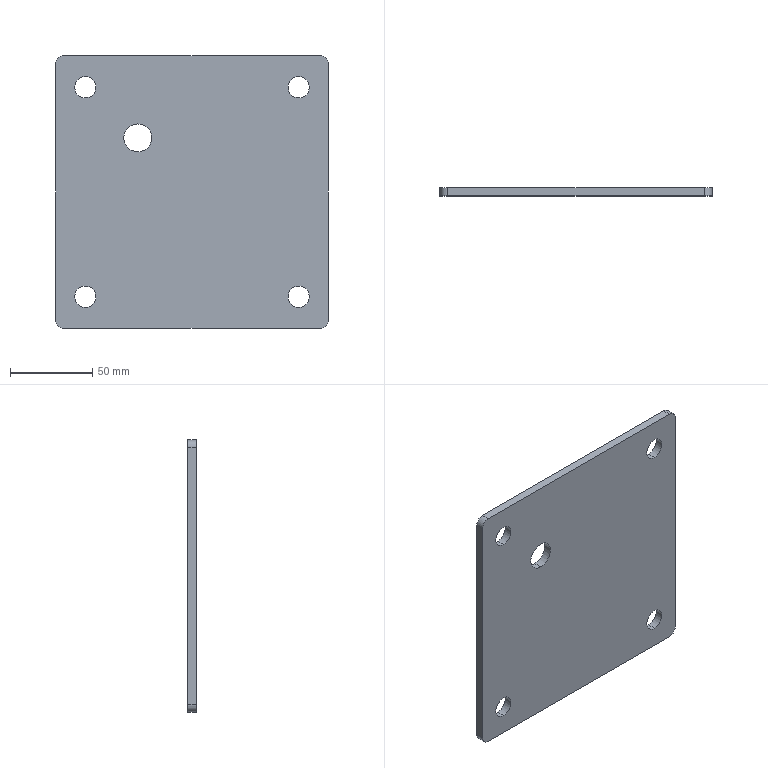Part | SolidWorks | features BaseBody 1 | 1 solid | 20 faces | box 166 x 5 x 166 mm | volume 133883 mm3 | cylinder 14 | plane 6 | commonest cylinder face diameters 13 x8 10 x4 17 x2
STEP:
#1=CARTESIAN_POINT('',(-33.,0.,24.5));
#2=VERTEX_POINT('',#1);
#3=CARTESIAN_POINT('',(-33.,0.,41.5));
#4=VERTEX_POINT('',#3);
#5=CARTESIAN_POINT('',(-33.,0.,33.));
#6=DIRECTION('',(0.,1.,0.));
#7=DIRECTION('',(0.,0.,1.));
#8=AXIS2_PLACEMENT_3D('',#5,#6,#7);
#9=CIRCLE('',#8,8.5);
#10=EDGE_CURVE('',#2,#4,#9,.T.);
#11=ORIENTED_EDGE('',*,*,#10,.F.);
#12=CARTESIAN_POINT('',(-33.,5.,24.5));
#13=VERTEX_POINT('',#12);
#14=CARTESIAN_POINT('',(-33.,1.,24.5));
#15=DIRECTION('',(0.,1.,0.));
#16=VECTOR('',#15,1000.);
#17=LINE('',#14,#16);
#18=EDGE_CURVE('',#2,#13,#17,.T.);
#19=ORIENTED_EDGE('',*,*,#18,.T.);
#20=CARTESIAN_POINT('',(-33.,5.,41.5));
#21=VERTEX_POINT('',#20);
#22=CARTESIAN_POINT('',(-33.,5.,33.));
#23=DIRECTION('',(0.,-1.,0.));
#24=DIRECTION('',(0.,0.,1.));
#25=AXIS2_PLACEMENT_3D('',#22,#23,#24);
#26=CIRCLE('',#25,8.5);
#27=EDGE_CURVE('',#21,#13,#26,.T.);
#28=ORIENTED_EDGE('',*,*,#27,.F.);
#29=CARTESIAN_POINT('',(-33.,1.,41.5));
#30=DIRECTION('',(0.,1.,0.));
#31=VECTOR('',#30,1000.);
#32=LINE('',#29,#31);
#33=EDGE_CURVE('',#4,#21,#32,.T.);
#34=ORIENTED_EDGE('',*,*,#33,.F.);
#35=EDGE_LOOP('',(#11,#19,#28,#34));
#36=FACE_OUTER_BOUND('',#35,.T.);
#37=CARTESIAN_POINT('',(-33.,1.,33.));
#38=DIRECTION('',(0.,1.,0.));
#39=DIRECTION('',(0.,0.,1.));
#40=AXIS2_PLACEMENT_3D('',#37,#38,#39);
#41=CYLINDRICAL_SURFACE('',#40,8.5);
#42=ADVANCED_FACE('',(#36),#41,.F.);
#43=CARTESIAN_POINT('',(-65.,0.,-70.262));
#44=VERTEX_POINT('',#43);
#45=CARTESIAN_POINT('',(-65.,0.,-57.262));
#46=VERTEX_POINT('',#45);
#47=CARTESIAN_POINT('',(-65.,0.,-63.762));
#48=DIRECTION('',(0.,1.,0.));
#49=DIRECTION('',(0.,0.,1.));
#50=AXIS2_PLACEMENT_3D('',#47,#48,#49);
#51=CIRCLE('',#50,6.5);
#52=EDGE_CURVE('',#44,#46,#51,.T.);
#53=ORIENTED_EDGE('',*,*,#52,.F.);
#54=CARTESIAN_POINT('',(-65.,5.,-70.262));
#55=VERTEX_POINT('',#54);
#56=CARTESIAN_POINT('',(-65.,-229.813,-70.262));
#57=DIRECTION('',(0.,1.,0.));
#58=VECTOR('',#57,1000.);
#59=LINE('',#56,#58);
#60=EDGE_CURVE('',#44,#55,#59,.T.);
#61=ORIENTED_EDGE('',*,*,#60,.T.);
#62=CARTESIAN_POINT('',(-65.,5.,-57.262));
#63=VERTEX_POINT('',#62);
#64=CARTESIAN_POINT('',(-65.,5.,-63.762));
#65=DIRECTION('',(0.,-1.,0.));
#66=DIRECTION('',(0.,0.,1.));
#67=AXIS2_PLACEMENT_3D('',#64,#65,#66);
#68=CIRCLE('',#67,6.5);
#69=EDGE_CURVE('',#63,#55,#68,.T.);
#70=ORIENTED_EDGE('',*,*,#69,.F.);
#71=CARTESIAN_POINT('',(-65.,-229.813,-57.262));
#72=DIRECTION('',(0.,1.,0.));
#73=VECTOR('',#72,1000.);
#74=LINE('',#71,#73);
#75=EDGE_CURVE('',#46,#63,#74,.T.);
#76=ORIENTED_EDGE('',*,*,#75,.F.);
#77=EDGE_LOOP('',(#53,#61,#70,#76));
#78=FACE_OUTER_BOUND('',#77,.T.);
#79=CARTESIAN_POINT('',(-65.,-229.813,-63.762));
#80=DIRECTION('',(0.,1.,0.));
#81=DIRECTION('',(0.,0.,1.));
#82=AXIS2_PLACEMENT_3D('',#79,#80,#81);
#83=CYLINDRICAL_SURFACE('',#82,6.5);
#84=ADVANCED_FACE('',(#78),#83,.F.);
#85=CARTESIAN_POINT('',(65.,0.,57.262));
#86=VERTEX_POINT('',#85);
#87=CARTESIAN_POINT('',(65.,0.,70.262));
#88=VERTEX_POINT('',#87);
#89=CARTESIAN_POINT('',(65.,0.,63.762));
#90=DIRECTION('',(0.,1.,0.));
#91=DIRECTION('',(0.,0.,1.));
#92=AXIS2_PLACEMENT_3D('',#89,#90,#91);
#93=CIRCLE('',#92,6.5);
#94=EDGE_CURVE('',#86,#88,#93,.T.);
#95=ORIENTED_EDGE('',*,*,#94,.F.);
#96=CARTESIAN_POINT('',(65.,5.,57.262));
#97=VERTEX_POINT('',#96);
#98=CARTESIAN_POINT('',(65.,-229.813,57.262));
#99=DIRECTION('',(0.,1.,0.));
#100=VECTOR('',#99,1000.);
#101=LINE('',#98,#100);
#102=EDGE_CURVE('',#86,#97,#101,.T.);
#103=ORIENTED_EDGE('',*,*,#102,.T.);
#104=CARTESIAN_POINT('',(65.,5.,70.262));
#105=VERTEX_POINT('',#104);
#106=CARTESIAN_POINT('',(65.,5.,63.762));
#107=DIRECTION('',(0.,-1.,0.));
#108=DIRECTION('',(0.,0.,1.));
#109=AXIS2_PLACEMENT_3D('',#106,#107,#108);
#110=CIRCLE('',#109,6.5);
#111=EDGE_CURVE('',#105,#97,#110,.T.);
#112=ORIENTED_EDGE('',*,*,#111,.F.);
#113=CARTESIAN_POINT('',(65.,-229.813,70.262));
#114=DIRECTION('',(0.,1.,0.));
#115=VECTOR('',#114,1000.);
#116=LINE('',#113,#115);
#117=EDGE_CURVE('',#88,#105,#116,.T.);
#118=ORIENTED_EDGE('',*,*,#117,.F.);
#119=EDGE_LOOP('',(#95,#103,#112,#118));
#120=FACE_OUTER_BOUND('',#119,.T.);
#121=CARTESIAN_POINT('',(65.,-229.813,63.762));
#122=DIRECTION('',(0.,1.,0.));
#123=DIRECTION('',(0.,0.,1.));
#124=AXIS2_PLACEMENT_3D('',#121,#122,#123);
#125=CYLINDRICAL_SURFACE('',#124,6.5);
#126=ADVANCED_FACE('',(#120),#125,.F.);
#127=CARTESIAN_POINT('',(65.,0.,-70.262));
#128=VERTEX_POINT('',#127);
#129=CARTESIAN_POINT('',(65.,0.,-57.262));
#130=VERTEX_POINT('',#129);
#131=CARTESIAN_POINT('',(65.,0.,-63.762));
#132=DIRECTION('',(0.,1.,0.));
#133=DIRECTION('',(0.,0.,1.));
#134=AXIS2_PLACEMENT_3D('',#131,#132,#133);
#135=CIRCLE('',#134,6.5);
#136=EDGE_CURVE('',#128,#130,#135,.T.);
#137=ORIENTED_EDGE('',*,*,#136,.F.);
#138=CARTESIAN_POINT('',(65.,5.,-70.262));
#139=VERTEX_POINT('',#138);
#140=CARTESIAN_POINT('',(65.,-229.813,-70.262));
#141=DIRECTION('',(0.,1.,0.));
#142=VECTOR('',#141,1000.);
#143=LINE('',#140,#142);
#144=EDGE_CURVE('',#128,#139,#143,.T.);
#145=ORIENTED_EDGE('',*,*,#144,.T.);
#146=CARTESIAN_POINT('',(65.,5.,-57.262));
#147=VERTEX_POINT('',#146);
#148=CARTESIAN_POINT('',(65.,5.,-63.762));
#149=DIRECTION('',(0.,-1.,0.));
#150=DIRECTION('',(0.,0.,1.));
#151=AXIS2_PLACEMENT_3D('',#148,#149,#150);
#152=CIRCLE('',#151,6.5);
#153=EDGE_CURVE('',#147,#139,#152,.T.);
#154=ORIENTED_EDGE('',*,*,#153,.F.);
#155=CARTESIAN_POINT('',(65.,-229.813,-57.262));
#156=DIRECTION('',(0.,1.,0.));
#157=VECTOR('',#156,1000.);
#158=LINE('',#155,#157);
#159=EDGE_CURVE('',#130,#147,#158,.T.);
#160=ORIENTED_EDGE('',*,*,#159,.F.);
#161=EDGE_LOOP('',(#137,#145,#154,#160));
#162=FACE_OUTER_BOUND('',#161,.T.);
#163=CARTESIAN_POINT('',(65.,-229.813,-63.762));
#164=DIRECTION('',(0.,1.,0.));
#165=DIRECTION('',(0.,0.,1.));
#166=AXIS2_PLACEMENT_3D('',#163,#164,#165);
#167=CYLINDRICAL_SURFACE('',#166,6.5);
#168=ADVANCED_FACE('',(#162),#167,.F.);
#169=CARTESIAN_POINT('',(-65.,0.,57.262));
#170=VERTEX_POINT('',#169);
#171=CARTESIAN_POINT('',(-65.,0.,70.262));
#172=VERTEX_POINT('',#171);
#173=CARTESIAN_POINT('',(-65.,0.,63.762));
#174=DIRECTION('',(0.,1.,0.));
#175=DIRECTION('',(0.,0.,1.));
#176=AXIS2_PLACEMENT_3D('',#173,#174,#175);
#177=CIRCLE('',#176,6.5);
#178=EDGE_CURVE('',#170,#172,#177,.T.);
#179=ORIENTED_EDGE('',*,*,#178,.F.);
#180=CARTESIAN_POINT('',(-65.,5.,57.262));
#181=VERTEX_POINT('',#180);
#182=CARTESIAN_POINT('',(-65.,-229.813,57.262));
#183=DIRECTION('',(0.,1.,0.));
#184=VECTOR('',#183,1000.);
#185=LINE('',#182,#184);
#186=EDGE_CURVE('',#170,#181,#185,.T.);
#187=ORIENTED_EDGE('',*,*,#186,.T.);
#188=CARTESIAN_POINT('',(-65.,5.,70.262));
#189=VERTEX_POINT('',#188);
#190=CARTESIAN_POINT('',(-65.,5.,63.762));
#191=DIRECTION('',(0.,-1.,0.));
#192=DIRECTION('',(0.,0.,1.));
#193=AXIS2_PLACEMENT_3D('',#190,#191,#192);
#194=CIRCLE('',#193,6.5);
#195=EDGE_CURVE('',#189,#181,#194,.T.);
#196=ORIENTED_EDGE('',*,*,#195,.F.);
#197=CARTESIAN_POINT('',(-65.,-229.813,70.262));
#198=DIRECTION('',(0.,1.,0.));
#199=VECTOR('',#198,1000.);
#200=LINE('',#197,#199);
#201=EDGE_CURVE('',#172,#189,#200,.T.);
#202=ORIENTED_EDGE('',*,*,#201,.F.);
#203=EDGE_LOOP('',(#179,#187,#196,#202));
#204=FACE_OUTER_BOUND('',#203,.T.);
#205=CARTESIAN_POINT('',(-65.,-229.813,63.762));
#206=DIRECTION('',(0.,1.,0.));
#207=DIRECTION('',(0.,0.,1.));
#208=AXIS2_PLACEMENT_3D('',#205,#206,#207);
#209=CYLINDRICAL_SURFACE('',#208,6.5);
#210=ADVANCED_FACE('',(#204),#209,.F.);
#211=ORIENTED_EDGE('',*,*,#27,.T.);
#212=CARTESIAN_POINT('',(-33.,5.,33.));
#213=DIRECTION('',(0.,-1.,0.));
#214=DIRECTION('',(0.,0.,1.));
#215=AXIS2_PLACEMENT_3D('',#212,#213,#214);
#216=CIRCLE('',#215,8.5);
#217=EDGE_CURVE('',#13,#21,#216,.T.);
#218=ORIENTED_EDGE('',*,*,#217,.T.);
#219=EDGE_LOOP('',(#211,#218));
#220=FACE_BOUND('',#219,.T.);
#221=ORIENTED_EDGE('',*,*,#69,.T.);
#222=CARTESIAN_POINT('',(-65.,5.,-63.762));
#223=DIRECTION('',(0.,-1.,0.));
#224=DIRECTION('',(0.,0.,1.));
#225=AXIS2_PLACEMENT_3D('',#222,#223,#224);
#226=CIRCLE('',#225,6.5);
#227=EDGE_CURVE('',#55,#63,#226,.T.);
#228=ORIENTED_EDGE('',*,*,#227,.T.);
#229=EDGE_LOOP('',(#221,#228));
#230=FACE_BOUND('',#229,.T.);
#231=ORIENTED_EDGE('',*,*,#111,.T.);
#232=CARTESIAN_POINT('',(65.,5.,63.762));
#233=DIRECTION('',(0.,-1.,0.));
#234=DIRECTION('',(0.,0.,1.));
#235=AXIS2_PLACEMENT_3D('',#232,#233,#234);
#236=CIRCLE('',#235,6.5);
#237=EDGE_CURVE('',#97,#105,#236,.T.);
#238=ORIENTED_EDGE('',*,*,#237,.T.);
#239=EDGE_LOOP('',(#231,#238));
#240=FACE_BOUND('',#239,.T.);
#241=ORIENTED_EDGE('',*,*,#153,.T.);
#242=CARTESIAN_POINT('',(65.,5.,-63.762));
#243=DIRECTION('',(0.,-1.,0.));
#244=DIRECTION('',(0.,0.,1.));
#245=AXIS2_PLACEMENT_3D('',#242,#243,#244);
#246=CIRCLE('',#245,6.5);
#247=EDGE_CURVE('',#139,#147,#246,.T.);
#248=ORIENTED_EDGE('',*,*,#247,.T.);
#249=EDGE_LOOP('',(#241,#248));
#250=FACE_BOUND('',#249,.T.);
#251=ORIENTED_EDGE('',*,*,#195,.T.);
#252=CARTESIAN_POINT('',(-65.,5.,63.762));
#253=DIRECTION('',(0.,-1.,0.));
#254=DIRECTION('',(0.,0.,1.));
#255=AXIS2_PLACEMENT_3D('',#252,#253,#254);
#256=CIRCLE('',#255,6.5);
#257=EDGE_CURVE('',#181,#189,#256,.T.);
#258=ORIENTED_EDGE('',*,*,#257,.T.);
#259=EDGE_LOOP('',(#251,#258));
#260=FACE_BOUND('',#259,.T.);
#261=CARTESIAN_POINT('',(-78.,5.,-83.));
#262=VERTEX_POINT('',#261);
#263=CARTESIAN_POINT('',(-83.,5.,-78.));
#264=VERTEX_POINT('',#263);
#265=CARTESIAN_POINT('',(-78.,5.,-78.));
#266=DIRECTION('',(0.,1.,0.));
#267=DIRECTION('',(0.,0.,1.));
#268=AXIS2_PLACEMENT_3D('',#265,#266,#267);
#269=CIRCLE('',#268,5.);
#270=EDGE_CURVE('',#262,#264,#269,.T.);
#271=ORIENTED_EDGE('',*,*,#270,.T.);
#272=CARTESIAN_POINT('',(-83.,5.,78.));
#273=VERTEX_POINT('',#272);
#274=CARTESIAN_POINT('',(-83.,5.,0.));
#275=DIRECTION('',(0.,0.,1.));
#276=VECTOR('',#275,1000.);
#277=LINE('',#274,#276);
#278=EDGE_CURVE('',#264,#273,#277,.T.);
#279=ORIENTED_EDGE('',*,*,#278,.T.);
#280=CARTESIAN_POINT('',(-78.,5.,83.));
#281=VERTEX_POINT('',#280);
#282=CARTESIAN_POINT('',(-78.,5.,78.));
#283=DIRECTION('',(0.,1.,0.));
#284=DIRECTION('',(0.,0.,1.));
#285=AXIS2_PLACEMENT_3D('',#282,#283,#284);
#286=CIRCLE('',#285,5.);
#287=EDGE_CURVE('',#273,#281,#286,.T.);
#288=ORIENTED_EDGE('',*,*,#287,.T.);
#289=CARTESIAN_POINT('',(78.,5.,83.));
#290=VERTEX_POINT('',#289);
#291=CARTESIAN_POINT('',(0.,5.,83.));
#292=DIRECTION('',(1.,0.,0.));
#293=VECTOR('',#292,1000.);
#294=LINE('',#291,#293);
#295=EDGE_CURVE('',#281,#290,#294,.T.);
#296=ORIENTED_EDGE('',*,*,#295,.T.);
#297=CARTESIAN_POINT('',(83.,5.,78.));
#298=VERTEX_POINT('',#297);
#299=CARTESIAN_POINT('',(78.,5.,78.));
#300=DIRECTION('',(0.,1.,0.));
#301=DIRECTION('',(0.,0.,1.));
#302=AXIS2_PLACEMENT_3D('',#299,#300,#301);
#303=CIRCLE('',#302,5.);
#304=EDGE_CURVE('',#290,#298,#303,.T.);
#305=ORIENTED_EDGE('',*,*,#304,.T.);
#306=CARTESIAN_POINT('',(83.,5.,-78.));
#307=VERTEX_POINT('',#306);
#308=CARTESIAN_POINT('',(83.,5.,0.));
#309=DIRECTION('',(0.,0.,-1.));
#310=VECTOR('',#309,1000.);
#311=LINE('',#308,#310);
#312=EDGE_CURVE('',#298,#307,#311,.T.);
#313=ORIENTED_EDGE('',*,*,#312,.T.);
#314=CARTESIAN_POINT('',(78.,5.,-83.));
#315=VERTEX_POINT('',#314);
#316=CARTESIAN_POINT('',(78.,5.,-78.));
#317=DIRECTION('',(0.,1.,0.));
#318=DIRECTION('',(0.,0.,1.));
#319=AXIS2_PLACEMENT_3D('',#316,#317,#318);
#320=CIRCLE('',#319,5.);
#321=EDGE_CURVE('',#307,#315,#320,.T.);
#322=ORIENTED_EDGE('',*,*,#321,.T.);
#323=CARTESIAN_POINT('',(0.,5.,-83.));
#324=DIRECTION('',(-1.,0.,0.));
#325=VECTOR('',#324,1000.);
#326=LINE('',#323,#325);
#327=EDGE_CURVE('',#315,#262,#326,.T.);
#328=ORIENTED_EDGE('',*,*,#327,.T.);
#329=EDGE_LOOP('',(#271,#279,#288,#296,#305,#313,#322,#328));
#330=FACE_OUTER_BOUND('',#329,.T.);
#331=CARTESIAN_POINT('',(0.,5.,0.));
#332=DIRECTION('',(0.,1.,0.));
#333=DIRECTION('',(0.,0.,1.));
#334=AXIS2_PLACEMENT_3D('',#331,#332,#333);
#335=PLANE('',#334);
#336=ADVANCED_FACE('',(#220,#230,#240,#250,#260,#330),#335,.T.);
#337=ORIENTED_EDGE('',*,*,#18,.F.);
#338=CARTESIAN_POINT('',(-33.,0.,33.));
#339=DIRECTION('',(0.,1.,0.));
#340=DIRECTION('',(0.,0.,1.));
#341=AXIS2_PLACEMENT_3D('',#338,#339,#340);
#342=CIRCLE('',#341,8.5);
#343=EDGE_CURVE('',#4,#2,#342,.T.);
#344=ORIENTED_EDGE('',*,*,#343,.F.);
#345=ORIENTED_EDGE('',*,*,#33,.T.);
#346=ORIENTED_EDGE('',*,*,#217,.F.);
#347=EDGE_LOOP('',(#337,#344,#345,#346));
#348=FACE_OUTER_BOUND('',#347,.T.);
#349=CARTESIAN_POINT('',(-33.,1.,33.));
#350=DIRECTION('',(0.,1.,0.));
#351=DIRECTION('',(0.,0.,1.));
#352=AXIS2_PLACEMENT_3D('',#349,#350,#351);
#353=CYLINDRICAL_SURFACE('',#352,8.5);
#354=ADVANCED_FACE('',(#348),#353,.F.);
#355=ORIENTED_EDGE('',*,*,#60,.F.);
#356=CARTESIAN_POINT('',(-65.,0.,-63.762));
#357=DIRECTION('',(0.,1.,0.));
#358=DIRECTION('',(0.,0.,1.));
#359=AXIS2_PLACEMENT_3D('',#356,#357,#358);
#360=CIRCLE('',#359,6.5);
#361=EDGE_CURVE('',#46,#44,#360,.T.);
#362=ORIENTED_EDGE('',*,*,#361,.F.);
#363=ORIENTED_EDGE('',*,*,#75,.T.);
#364=ORIENTED_EDGE('',*,*,#227,.F.);
#365=EDGE_LOOP('',(#355,#362,#363,#364));
#366=FACE_OUTER_BOUND('',#365,.T.);
#367=CARTESIAN_POINT('',(-65.,-229.813,-63.762));
#368=DIRECTION('',(0.,1.,0.));
#369=DIRECTION('',(0.,0.,1.));
#370=AXIS2_PLACEMENT_3D('',#367,#368,#369);
#371=CYLINDRICAL_SURFACE('',#370,6.5);
#372=ADVANCED_FACE('',(#366),#371,.F.);
#373=ORIENTED_EDGE('',*,*,#102,.F.);
#374=CARTESIAN_POINT('',(65.,0.,63.762));
#375=DIRECTION('',(0.,1.,0.));
#376=DIRECTION('',(0.,0.,1.));
#377=AXIS2_PLACEMENT_3D('',#374,#375,#376);
#378=CIRCLE('',#377,6.5);
#379=EDGE_CURVE('',#88,#86,#378,.T.);
#380=ORIENTED_EDGE('',*,*,#379,.F.);
#381=ORIENTED_EDGE('',*,*,#117,.T.);
#382=ORIENTED_EDGE('',*,*,#237,.F.);
#383=EDGE_LOOP('',(#373,#380,#381,#382));
#384=FACE_OUTER_BOUND('',#383,.T.);
#385=CARTESIAN_POINT('',(65.,-229.813,63.762));
#386=DIRECTION('',(0.,1.,0.));
#387=DIRECTION('',(0.,0.,1.));
#388=AXIS2_PLACEMENT_3D('',#385,#386,#387);
#389=CYLINDRICAL_SURFACE('',#388,6.5);
#390=ADVANCED_FACE('',(#384),#389,.F.);
#391=ORIENTED_EDGE('',*,*,#144,.F.);
#392=CARTESIAN_POINT('',(65.,0.,-63.762));
#393=DIRECTION('',(0.,1.,0.));
#394=DIRECTION('',(0.,0.,1.));
#395=AXIS2_PLACEMENT_3D('',#392,#393,#394);
#396=CIRCLE('',#395,6.5);
#397=EDGE_CURVE('',#130,#128,#396,.T.);
#398=ORIENTED_EDGE('',*,*,#397,.F.);
#399=ORIENTED_EDGE('',*,*,#159,.T.);
#400=ORIENTED_EDGE('',*,*,#247,.F.);
#401=EDGE_LOOP('',(#391,#398,#399,#400));
#402=FACE_OUTER_BOUND('',#401,.T.);
#403=CARTESIAN_POINT('',(65.,-229.813,-63.762));
#404=DIRECTION('',(0.,1.,0.));
#405=DIRECTION('',(0.,0.,1.));
#406=AXIS2_PLACEMENT_3D('',#403,#404,#405);
#407=CYLINDRICAL_SURFACE('',#406,6.5);
#408=ADVANCED_FACE('',(#402),#407,.F.);
#409=ORIENTED_EDGE('',*,*,#186,.F.);
#410=CARTESIAN_POINT('',(-65.,0.,63.762));
#411=DIRECTION('',(0.,1.,0.));
#412=DIRECTION('',(0.,0.,1.));
#413=AXIS2_PLACEMENT_3D('',#410,#411,#412);
#414=CIRCLE('',#413,6.5);
#415=EDGE_CURVE('',#172,#170,#414,.T.);
#416=ORIENTED_EDGE('',*,*,#415,.F.);
#417=ORIENTED_EDGE('',*,*,#201,.T.);
#418=ORIENTED_EDGE('',*,*,#257,.F.);
#419=EDGE_LOOP('',(#409,#416,#417,#418));
#420=FACE_OUTER_BOUND('',#419,.T.);
#421=CARTESIAN_POINT('',(-65.,-229.813,63.762));
#422=DIRECTION('',(0.,1.,0.));
#423=DIRECTION('',(0.,0.,1.));
#424=AXIS2_PLACEMENT_3D('',#421,#422,#423);
#425=CYLINDRICAL_SURFACE('',#424,6.5);
#426=ADVANCED_FACE('',(#420),#425,.F.);
#427=CARTESIAN_POINT('',(-83.,0.,-78.));
#428=VERTEX_POINT('',#427);
#429=CARTESIAN_POINT('',(-83.,0.,-78.));
#430=DIRECTION('',(0.,-1.,0.));
#431=VECTOR('',#430,1000.);
#432=LINE('',#429,#431);
#433=EDGE_CURVE('',#264,#428,#432,.T.);
#434=ORIENTED_EDGE('',*,*,#433,.T.);
#435=CARTESIAN_POINT('',(-83.,0.,78.));
#436=VERTEX_POINT('',#435);
#437=CARTESIAN_POINT('',(-83.,0.,-83.));
#438=DIRECTION('',(0.,0.,1.));
#439=VECTOR('',#438,1000.);
#440=LINE('',#437,#439);
#441=EDGE_CURVE('',#428,#436,#440,.T.);
#442=ORIENTED_EDGE('',*,*,#441,.T.);
#443=CARTESIAN_POINT('',(-83.,0.,78.));
#444=DIRECTION('',(0.,1.,0.));
#445=VECTOR('',#444,1000.);
#446=LINE('',#443,#445);
#447=EDGE_CURVE('',#436,#273,#446,.T.);
#448=ORIENTED_EDGE('',*,*,#447,.T.);
#449=ORIENTED_EDGE('',*,*,#278,.F.);
#450=EDGE_LOOP('',(#434,#442,#448,#449));
#451=FACE_OUTER_BOUND('',#450,.T.);
#452=CARTESIAN_POINT('',(-83.,0.,-83.));
#453=DIRECTION('',(-1.,0.,0.));
#454=DIRECTION('',(0.,0.,1.));
#455=AXIS2_PLACEMENT_3D('',#452,#453,#454);
#456=PLANE('',#455);
#457=ADVANCED_FACE('',(#451),#456,.T.);
#458=CARTESIAN_POINT('',(-78.,0.,-83.));
#459=VERTEX_POINT('',#458);
#460=CARTESIAN_POINT('',(-78.,0.,-78.));
#461=DIRECTION('',(0.,1.,0.));
#462=DIRECTION('',(0.,0.,1.));
#463=AXIS2_PLACEMENT_3D('',#460,#461,#462);
#464=CIRCLE('',#463,5.);
#465=EDGE_CURVE('',#459,#428,#464,.T.);
#466=ORIENTED_EDGE('',*,*,#465,.T.);
#467=ORIENTED_EDGE('',*,*,#433,.F.);
#468=ORIENTED_EDGE('',*,*,#270,.F.);
#469=CARTESIAN_POINT('',(-78.,0.,-83.));
#470=DIRECTION('',(0.,-1.,0.));
#471=VECTOR('',#470,1000.);
#472=LINE('',#469,#471);
#473=EDGE_CURVE('',#262,#459,#472,.T.);
#474=ORIENTED_EDGE('',*,*,#473,.T.);
#475=EDGE_LOOP('',(#466,#467,#468,#474));
#476=FACE_OUTER_BOUND('',#475,.T.);
#477=CARTESIAN_POINT('',(-78.,0.,-78.));
#478=DIRECTION('',(0.,1.,0.));
#479=DIRECTION('',(0.,0.,1.));
#480=AXIS2_PLACEMENT_3D('',#477,#478,#479);
#481=CYLINDRICAL_SURFACE('',#480,5.);
#482=ADVANCED_FACE('',(#476),#481,.T.);
#483=CARTESIAN_POINT('',(78.,0.,-83.));
#484=VERTEX_POINT('',#483);
#485=CARTESIAN_POINT('',(78.,0.,-83.));
#486=DIRECTION('',(0.,-1.,0.));
#487=VECTOR('',#486,1000.);
#488=LINE('',#485,#487);
#489=EDGE_CURVE('',#315,#484,#488,.T.);
#490=ORIENTED_EDGE('',*,*,#489,.T.);
#491=CARTESIAN_POINT('',(83.,0.,-83.));
#492=DIRECTION('',(-1.,0.,0.));
#493=VECTOR('',#492,1000.);
#494=LINE('',#491,#493);
#495=EDGE_CURVE('',#484,#459,#494,.T.);
#496=ORIENTED_EDGE('',*,*,#495,.T.);
#497=ORIENTED_EDGE('',*,*,#473,.F.);
#498=ORIENTED_EDGE('',*,*,#327,.F.);
#499=EDGE_LOOP('',(#490,#496,#497,#498));
#500=FACE_OUTER_BOUND('',#499,.T.);
#501=CARTESIAN_POINT('',(83.,0.,-83.));
#502=DIRECTION('',(0.,0.,-1.));
#503=DIRECTION('',(-1.,0.,0.));
#504=AXIS2_PLACEMENT_3D('',#501,#502,#503);
#505=PLANE('',#504);
#506=ADVANCED_FACE('',(#500),#505,.T.);
#507=CARTESIAN_POINT('',(83.,0.,-78.));
#508=VERTEX_POINT('',#507);
#509=CARTESIAN_POINT('',(78.,0.,-78.));
#510=DIRECTION('',(0.,1.,0.));
#511=DIRECTION('',(0.,0.,1.));
#512=AXIS2_PLACEMENT_3D('',#509,#510,#511);
#513=CIRCLE('',#512,5.);
#514=EDGE_CURVE('',#508,#484,#513,.T.);
#515=ORIENTED_EDGE('',*,*,#514,.T.);
#516=ORIENTED_EDGE('',*,*,#489,.F.);
#517=ORIENTED_EDGE('',*,*,#321,.F.);
#518=CARTESIAN_POINT('',(83.,0.,-78.));
#519=DIRECTION('',(0.,-1.,0.));
#520=VECTOR('',#519,1000.);
#521=LINE('',#518,#520);
#522=EDGE_CURVE('',#307,#508,#521,.T.);
#523=ORIENTED_EDGE('',*,*,#522,.T.);
#524=EDGE_LOOP('',(#515,#516,#517,#523));
#525=FACE_OUTER_BOUND('',#524,.T.);
#526=CARTESIAN_POINT('',(78.,0.,-78.));
#527=DIRECTION('',(0.,1.,0.));
#528=DIRECTION('',(0.,0.,1.));
#529=AXIS2_PLACEMENT_3D('',#526,#527,#528);
#530=CYLINDRICAL_SURFACE('',#529,5.);
#531=ADVANCED_FACE('',(#525),#530,.T.);
#532=CARTESIAN_POINT('',(83.,0.,78.));
#533=VERTEX_POINT('',#532);
#534=CARTESIAN_POINT('',(83.,0.,78.));
#535=DIRECTION('',(0.,-1.,0.));
#536=VECTOR('',#535,1000.);
#537=LINE('',#534,#536);
#538=EDGE_CURVE('',#298,#533,#537,.T.);
#539=ORIENTED_EDGE('',*,*,#538,.T.);
#540=CARTESIAN_POINT('',(83.,0.,83.));
#541=DIRECTION('',(0.,0.,-1.));
#542=VECTOR('',#541,1000.);
#543=LINE('',#540,#542);
#544=EDGE_CURVE('',#533,#508,#543,.T.);
#545=ORIENTED_EDGE('',*,*,#544,.T.);
#546=ORIENTED_EDGE('',*,*,#522,.F.);
#547=ORIENTED_EDGE('',*,*,#312,.F.);
#548=EDGE_LOOP('',(#539,#545,#546,#547));
#549=FACE_OUTER_BOUND('',#548,.T.);
#550=CARTESIAN_POINT('',(83.,0.,83.));
#551=DIRECTION('',(1.,0.,0.));
#552=DIRECTION('',(0.,0.,-1.));
#553=AXIS2_PLACEMENT_3D('',#550,#551,#552);
#554=PLANE('',#553);
#555=ADVANCED_FACE('',(#549),#554,.T.);
#556=CARTESIAN_POINT('',(78.,0.,83.));
#557=VERTEX_POINT('',#556);
#558=CARTESIAN_POINT('',(78.,0.,78.));
#559=DIRECTION('',(0.,1.,0.));
#560=DIRECTION('',(0.,0.,1.));
#561=AXIS2_PLACEMENT_3D('',#558,#559,#560);
#562=CIRCLE('',#561,5.);
#563=EDGE_CURVE('',#557,#533,#562,.T.);
#564=ORIENTED_EDGE('',*,*,#563,.T.);
#565=ORIENTED_EDGE('',*,*,#538,.F.);
#566=ORIENTED_EDGE('',*,*,#304,.F.);
#567=CARTESIAN_POINT('',(78.,0.,83.));
#568=DIRECTION('',(0.,-1.,0.));
#569=VECTOR('',#568,1000.);
#570=LINE('',#567,#569);
#571=EDGE_CURVE('',#290,#557,#570,.T.);
#572=ORIENTED_EDGE('',*,*,#571,.T.);
#573=EDGE_LOOP('',(#564,#565,#566,#572));
#574=FACE_OUTER_BOUND('',#573,.T.);
#575=CARTESIAN_POINT('',(78.,0.,78.));
#576=DIRECTION('',(0.,1.,0.));
#577=DIRECTION('',(0.,0.,1.));
#578=AXIS2_PLACEMENT_3D('',#575,#576,#577);
#579=CYLINDRICAL_SURFACE('',#578,5.);
#580=ADVANCED_FACE('',(#574),#579,.T.);
#581=ORIENTED_EDGE('',*,*,#571,.F.);
#582=ORIENTED_EDGE('',*,*,#295,.F.);
#583=CARTESIAN_POINT('',(-78.,0.,83.));
#584=VERTEX_POINT('',#583);
#585=CARTESIAN_POINT('',(-78.,0.,83.));
#586=DIRECTION('',(0.,-1.,0.));
#587=VECTOR('',#586,1000.);
#588=LINE('',#585,#587);
#589=EDGE_CURVE('',#281,#584,#588,.T.);
#590=ORIENTED_EDGE('',*,*,#589,.T.);
#591=CARTESIAN_POINT('',(-83.,0.,83.));
#592=DIRECTION('',(1.,0.,0.));
#593=VECTOR('',#592,1000.);
#594=LINE('',#591,#593);
#595=EDGE_CURVE('',#584,#557,#594,.T.);
#596=ORIENTED_EDGE('',*,*,#595,.T.);
#597=EDGE_LOOP('',(#581,#582,#590,#596));
#598=FACE_OUTER_BOUND('',#597,.T.);
#599=CARTESIAN_POINT('',(-83.,0.,83.));
#600=DIRECTION('',(0.,0.,1.));
#601=DIRECTION('',(1.,0.,0.));
#602=AXIS2_PLACEMENT_3D('',#599,#600,#601);
#603=PLANE('',#602);
#604=ADVANCED_FACE('',(#598),#603,.T.);
#605=CARTESIAN_POINT('',(-78.,0.,78.));
#606=DIRECTION('',(0.,1.,0.));
#607=DIRECTION('',(0.,0.,1.));
#608=AXIS2_PLACEMENT_3D('',#605,#606,#607);
#609=CIRCLE('',#608,5.);
#610=EDGE_CURVE('',#436,#584,#609,.T.);
#611=ORIENTED_EDGE('',*,*,#610,.T.);
#612=ORIENTED_EDGE('',*,*,#589,.F.);
#613=ORIENTED_EDGE('',*,*,#287,.F.);
#614=ORIENTED_EDGE('',*,*,#447,.F.);
#615=EDGE_LOOP('',(#611,#612,#613,#614));
#616=FACE_OUTER_BOUND('',#615,.T.);
#617=CARTESIAN_POINT('',(-78.,0.,78.));
#618=DIRECTION('',(0.,1.,0.));
#619=DIRECTION('',(0.,0.,1.));
#620=AXIS2_PLACEMENT_3D('',#617,#618,#619);
#621=CYLINDRICAL_SURFACE('',#620,5.);
#622=ADVANCED_FACE('',(#616),#621,.T.);
#623=ORIENTED_EDGE('',*,*,#343,.T.);
#624=ORIENTED_EDGE('',*,*,#10,.T.);
#625=EDGE_LOOP('',(#623,#624));
#626=FACE_BOUND('',#625,.T.);
#627=ORIENTED_EDGE('',*,*,#361,.T.);
#628=ORIENTED_EDGE('',*,*,#52,.T.);
#629=EDGE_LOOP('',(#627,#628));
#630=FACE_BOUND('',#629,.T.);
#631=ORIENTED_EDGE('',*,*,#379,.T.);
#632=ORIENTED_EDGE('',*,*,#94,.T.);
#633=EDGE_LOOP('',(#631,#632));
#634=FACE_BOUND('',#633,.T.);
#635=ORIENTED_EDGE('',*,*,#397,.T.);
#636=ORIENTED_EDGE('',*,*,#136,.T.);
#637=EDGE_LOOP('',(#635,#636));
#638=FACE_BOUND('',#637,.T.);
#639=ORIENTED_EDGE('',*,*,#415,.T.);
#640=ORIENTED_EDGE('',*,*,#178,.T.);
#641=EDGE_LOOP('',(#639,#640));
#642=FACE_BOUND('',#641,.T.);
#643=ORIENTED_EDGE('',*,*,#563,.F.);
#644=ORIENTED_EDGE('',*,*,#595,.F.);
#645=ORIENTED_EDGE('',*,*,#610,.F.);
#646=ORIENTED_EDGE('',*,*,#441,.F.);
#647=ORIENTED_EDGE('',*,*,#465,.F.);
#648=ORIENTED_EDGE('',*,*,#495,.F.);
#649=ORIENTED_EDGE('',*,*,#514,.F.);
#650=ORIENTED_EDGE('',*,*,#544,.F.);
#651=EDGE_LOOP('',(#643,#644,#645,#646,#647,#648,#649,#650));
#652=FACE_OUTER_BOUND('',#651,.T.);
#653=CARTESIAN_POINT('',(0.,0.,0.));
#654=DIRECTION('',(0.,-1.,0.));
#655=DIRECTION('',(0.,0.,-1.));
#656=AXIS2_PLACEMENT_3D('',#653,#654,#655);
#657=PLANE('',#656);
#658=ADVANCED_FACE('',(#626,#630,#634,#638,#642,#652),#657,.T.);
#659=CLOSED_SHELL('',(#42,#84,#126,#168,#210,#336,#354,#372,#390,#408,#426,#457,#482,#506,#531,#555,#580,#604,#622,#658));
#660=MANIFOLD_SOLID_BREP('',#659);
#661=CARTESIAN_POINT('',(0.,0.,0.));
#662=DIRECTION('',(0.,0.,1.));
#663=DIRECTION('',(1.,0.,0.));
#664=AXIS2_PLACEMENT_3D('',#661,#662,#663);
#665=(LENGTH_UNIT()NAMED_UNIT(*)SI_UNIT(.MILLI.,.METRE.));
#666=UNCERTAINTY_MEASURE_WITH_UNIT(LENGTH_MEASURE(0.00001),#665,'','');
#667=(NAMED_UNIT(*)PLANE_ANGLE_UNIT()SI_UNIT($,.RADIAN.));
#668=(NAMED_UNIT(*)SI_UNIT($,.STERADIAN.)SOLID_ANGLE_UNIT());
#669=(GEOMETRIC_REPRESENTATION_CONTEXT(3)GLOBAL_UNCERTAINTY_ASSIGNED_CONTEXT((#666))GLOBAL_UNIT_ASSIGNED_CONTEXT((#665,#667,#668))REPRESENTATION_CONTEXT('',''));
#670=ADVANCED_BREP_SHAPE_REPRESENTATION('',(#660,#664),#669);